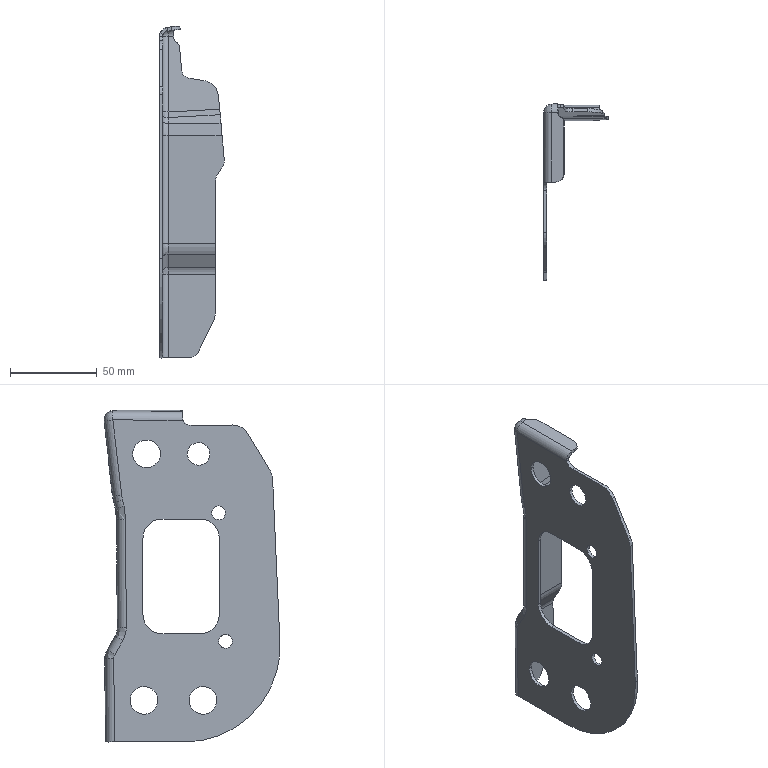Part | 1 solid | 108 faces | box 37.255 x 101.381 x 191.221 mm | volume 33091 mm3 | spline 46 | cylinder 43 | plane 15 | other 2 | sphere 2 | commonest cylinder face diameters 10 x8 6.4 x7 16 x6 8 x4 20 x4 22 x4